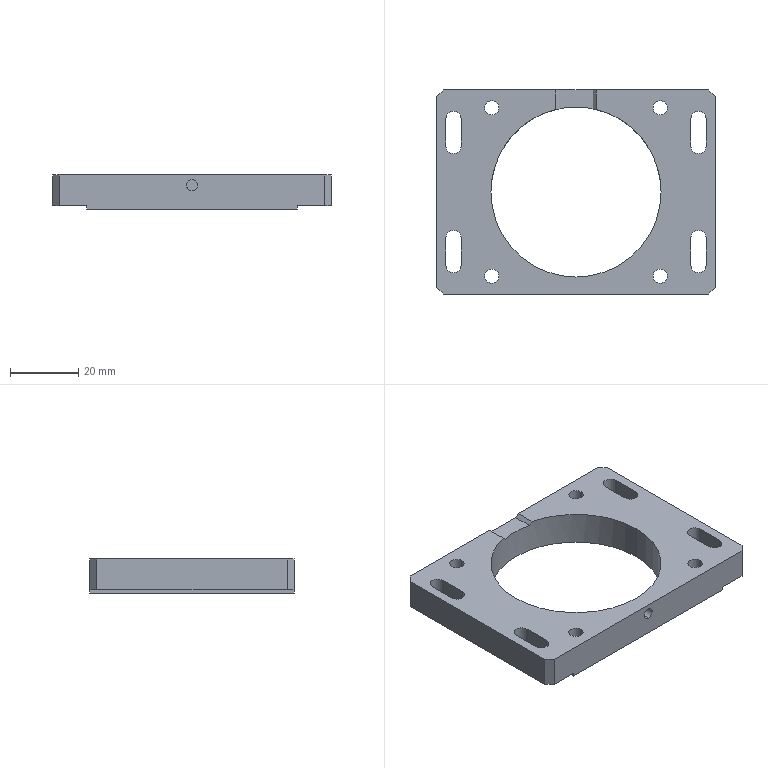Part | SolidWorks | features ICE 4, Chamfer 2, HoleWzd 2, Extrusion 1 | 1 solid | 45 faces | box 82 x 60 x 10 mm | volume 25770 mm3 | plane 25 | cylinder 20 | commonest cylinder face diameters 4.2 x8 4.5 x8 3.3 x2 50 x2